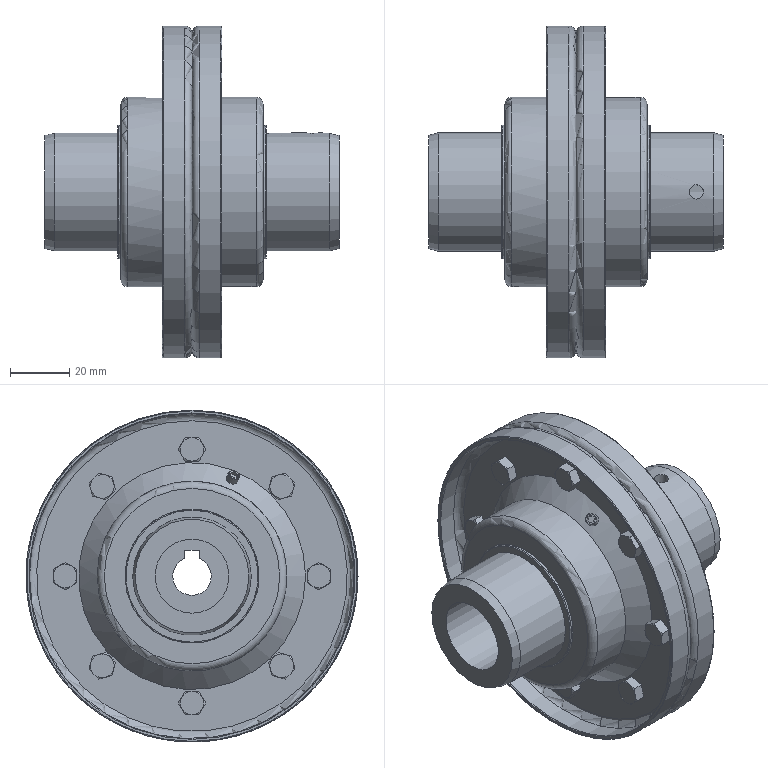Part | STEP file | couplings_22222 | 1 solid | 411 faces | box 99.2 x 112 x 112 mm | volume 164503 mm3 | plane 174 | cone 155 | cylinder 51 | torus 31 | commonest cylinder face diameters 5 x24 45.2 x6 40 x4 13 x2 55.2 x2 61.6 x2